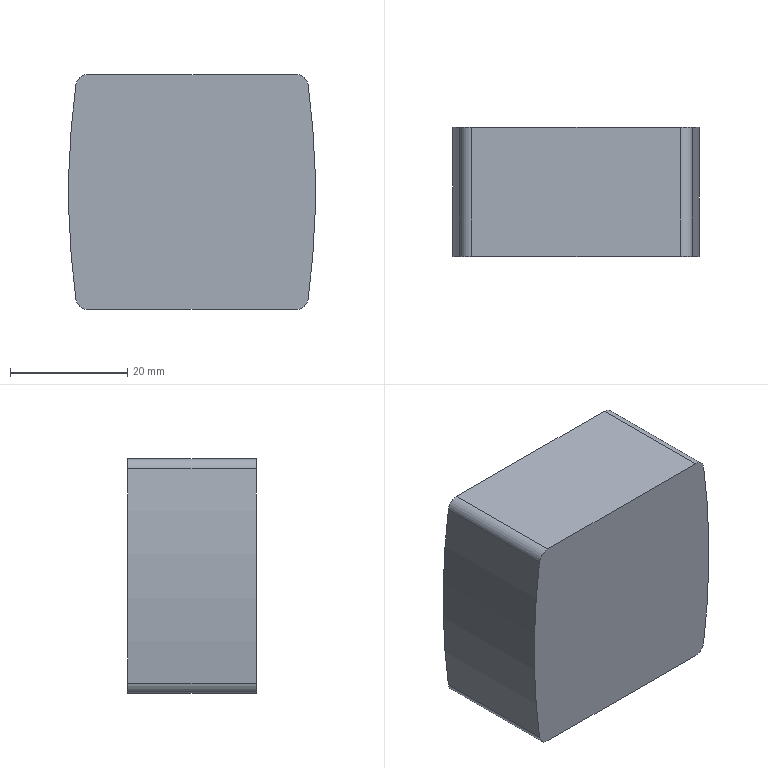Part | SolidWorks | features BaseBody 1 | 1 solid | 12 faces | box 42.009 x 21.95 x 40 mm | volume 35954 mm3 | cylinder 8 | plane 4 | commonest cylinder face diameters 4 x6 268.2 x2
STEP:
#1=CARTESIAN_POINT('',(17.75,69.98,-20.));
#2=VERTEX_POINT('',#1);
#3=CARTESIAN_POINT('',(17.773,69.98,-20.));
#4=VERTEX_POINT('',#3);
#5=CARTESIAN_POINT('',(17.773,69.98,-18.));
#6=DIRECTION('',(0.,-1.,0.));
#7=DIRECTION('',(0.,0.,-1.));
#8=AXIS2_PLACEMENT_3D('',#5,#6,#7);
#9=CIRCLE('',#8,2.);
#10=EDGE_CURVE('',#2,#4,#9,.T.);
#11=ORIENTED_EDGE('',*,*,#10,.T.);
#12=CARTESIAN_POINT('',(17.773,48.03,-20.));
#13=VERTEX_POINT('',#12);
#14=CARTESIAN_POINT('',(17.773,69.98,-20.));
#15=DIRECTION('',(0.,-1.,0.));
#16=VECTOR('',#15,1000.);
#17=LINE('',#14,#16);
#18=EDGE_CURVE('',#4,#13,#17,.T.);
#19=ORIENTED_EDGE('',*,*,#18,.T.);
#20=CARTESIAN_POINT('',(17.75,48.03,-20.));
#21=VERTEX_POINT('',#20);
#22=CARTESIAN_POINT('',(17.773,48.03,-18.));
#23=DIRECTION('',(0.,-1.,0.));
#24=DIRECTION('',(0.,0.,-1.));
#25=AXIS2_PLACEMENT_3D('',#22,#23,#24);
#26=CIRCLE('',#25,2.);
#27=EDGE_CURVE('',#21,#13,#26,.T.);
#28=ORIENTED_EDGE('',*,*,#27,.F.);
#29=CARTESIAN_POINT('',(17.75,69.98,-20.));
#30=DIRECTION('',(0.,1.,0.));
#31=VECTOR('',#30,1000.);
#32=LINE('',#29,#31);
#33=EDGE_CURVE('',#21,#2,#32,.T.);
#34=ORIENTED_EDGE('',*,*,#33,.T.);
#35=EDGE_LOOP('',(#11,#19,#28,#34));
#36=FACE_OUTER_BOUND('',#35,.T.);
#37=CARTESIAN_POINT('',(17.773,69.98,-18.));
#38=DIRECTION('',(0.,-1.,0.));
#39=DIRECTION('',(0.,0.,-1.));
#40=AXIS2_PLACEMENT_3D('',#37,#38,#39);
#41=CYLINDRICAL_SURFACE('',#40,2.);
#42=ADVANCED_FACE('',(#36),#41,.T.);
#43=CARTESIAN_POINT('',(-19.75,69.98,-18.3));
#44=VERTEX_POINT('',#43);
#45=CARTESIAN_POINT('',(-17.773,69.98,-20.));
#46=VERTEX_POINT('',#45);
#47=CARTESIAN_POINT('',(-17.773,69.98,-18.));
#48=DIRECTION('',(0.,-1.,0.));
#49=DIRECTION('',(0.,0.,-1.));
#50=AXIS2_PLACEMENT_3D('',#47,#48,#49);
#51=CIRCLE('',#50,2.);
#52=EDGE_CURVE('',#44,#46,#51,.T.);
#53=ORIENTED_EDGE('',*,*,#52,.T.);
#54=CARTESIAN_POINT('',(-17.773,48.03,-20.));
#55=VERTEX_POINT('',#54);
#56=CARTESIAN_POINT('',(-17.773,69.98,-20.));
#57=DIRECTION('',(0.,-1.,0.));
#58=VECTOR('',#57,1000.);
#59=LINE('',#56,#58);
#60=EDGE_CURVE('',#46,#55,#59,.T.);
#61=ORIENTED_EDGE('',*,*,#60,.T.);
#62=CARTESIAN_POINT('',(-19.75,48.03,-18.3));
#63=VERTEX_POINT('',#62);
#64=CARTESIAN_POINT('',(-17.773,48.03,-18.));
#65=DIRECTION('',(0.,-1.,0.));
#66=DIRECTION('',(0.,0.,-1.));
#67=AXIS2_PLACEMENT_3D('',#64,#65,#66);
#68=CIRCLE('',#67,2.);
#69=EDGE_CURVE('',#63,#55,#68,.T.);
#70=ORIENTED_EDGE('',*,*,#69,.F.);
#71=CARTESIAN_POINT('',(-19.75,69.98,-18.3));
#72=DIRECTION('',(0.,1.,0.));
#73=VECTOR('',#72,1000.);
#74=LINE('',#71,#73);
#75=EDGE_CURVE('',#63,#44,#74,.T.);
#76=ORIENTED_EDGE('',*,*,#75,.T.);
#77=EDGE_LOOP('',(#53,#61,#70,#76));
#78=FACE_OUTER_BOUND('',#77,.T.);
#79=CARTESIAN_POINT('',(-17.773,69.98,-18.));
#80=DIRECTION('',(0.,-1.,0.));
#81=DIRECTION('',(0.,0.,-1.));
#82=AXIS2_PLACEMENT_3D('',#79,#80,#81);
#83=CYLINDRICAL_SURFACE('',#82,2.);
#84=ADVANCED_FACE('',(#78),#83,.T.);
#85=CARTESIAN_POINT('',(19.75,48.03,-18.3));
#86=VERTEX_POINT('',#85);
#87=CARTESIAN_POINT('',(19.75,48.03,18.3));
#88=VERTEX_POINT('',#87);
#89=CARTESIAN_POINT('',(-113.095,48.03,0.));
#90=DIRECTION('',(0.,-1.,0.));
#91=DIRECTION('',(0.,0.,-1.));
#92=AXIS2_PLACEMENT_3D('',#89,#90,#91);
#93=CIRCLE('',#92,134.1);
#94=EDGE_CURVE('',#86,#88,#93,.T.);
#95=ORIENTED_EDGE('',*,*,#94,.T.);
#96=CARTESIAN_POINT('',(17.75,48.03,20.));
#97=VERTEX_POINT('',#96);
#98=CARTESIAN_POINT('',(17.773,48.03,18.));
#99=DIRECTION('',(0.,-1.,0.));
#100=DIRECTION('',(0.,0.,-1.));
#101=AXIS2_PLACEMENT_3D('',#98,#99,#100);
#102=CIRCLE('',#101,2.);
#103=EDGE_CURVE('',#88,#97,#102,.T.);
#104=ORIENTED_EDGE('',*,*,#103,.T.);
#105=CARTESIAN_POINT('',(-17.75,48.03,20.));
#106=VERTEX_POINT('',#105);
#107=CARTESIAN_POINT('',(0.,48.03,20.));
#108=DIRECTION('',(-1.,0.,0.));
#109=VECTOR('',#108,1000.);
#110=LINE('',#107,#109);
#111=EDGE_CURVE('',#97,#106,#110,.T.);
#112=ORIENTED_EDGE('',*,*,#111,.T.);
#113=CARTESIAN_POINT('',(-19.75,48.03,18.3));
#114=VERTEX_POINT('',#113);
#115=CARTESIAN_POINT('',(-17.773,48.03,18.));
#116=DIRECTION('',(0.,-1.,0.));
#117=DIRECTION('',(0.,0.,-1.));
#118=AXIS2_PLACEMENT_3D('',#115,#116,#117);
#119=CIRCLE('',#118,2.);
#120=EDGE_CURVE('',#106,#114,#119,.T.);
#121=ORIENTED_EDGE('',*,*,#120,.T.);
#122=CARTESIAN_POINT('',(113.095,48.03,0.));
#123=DIRECTION('',(0.,-1.,0.));
#124=DIRECTION('',(0.,0.,-1.));
#125=AXIS2_PLACEMENT_3D('',#122,#123,#124);
#126=CIRCLE('',#125,134.1);
#127=EDGE_CURVE('',#114,#63,#126,.T.);
#128=ORIENTED_EDGE('',*,*,#127,.T.);
#129=ORIENTED_EDGE('',*,*,#69,.T.);
#130=CARTESIAN_POINT('',(-17.75,48.03,-20.));
#131=VERTEX_POINT('',#130);
#132=CARTESIAN_POINT('',(-17.773,48.03,-18.));
#133=DIRECTION('',(0.,-1.,0.));
#134=DIRECTION('',(0.,0.,-1.));
#135=AXIS2_PLACEMENT_3D('',#132,#133,#134);
#136=CIRCLE('',#135,2.);
#137=EDGE_CURVE('',#55,#131,#136,.T.);
#138=ORIENTED_EDGE('',*,*,#137,.T.);
#139=CARTESIAN_POINT('',(0.,48.03,-20.));
#140=DIRECTION('',(1.,0.,0.));
#141=VECTOR('',#140,1000.);
#142=LINE('',#139,#141);
#143=EDGE_CURVE('',#131,#21,#142,.T.);
#144=ORIENTED_EDGE('',*,*,#143,.T.);
#145=ORIENTED_EDGE('',*,*,#27,.T.);
#146=CARTESIAN_POINT('',(17.773,48.03,-18.));
#147=DIRECTION('',(0.,-1.,0.));
#148=DIRECTION('',(0.,0.,-1.));
#149=AXIS2_PLACEMENT_3D('',#146,#147,#148);
#150=CIRCLE('',#149,2.);
#151=EDGE_CURVE('',#13,#86,#150,.T.);
#152=ORIENTED_EDGE('',*,*,#151,.T.);
#153=EDGE_LOOP('',(#95,#104,#112,#121,#128,#129,#138,#144,#145,#152));
#154=FACE_OUTER_BOUND('',#153,.T.);
#155=CARTESIAN_POINT('',(0.,48.03,0.));
#156=DIRECTION('',(0.,-1.,0.));
#157=DIRECTION('',(0.,0.,-1.));
#158=AXIS2_PLACEMENT_3D('',#155,#156,#157);
#159=PLANE('',#158);
#160=ADVANCED_FACE('',(#154),#159,.T.);
#161=CARTESIAN_POINT('',(19.75,69.98,18.3));
#162=VERTEX_POINT('',#161);
#163=CARTESIAN_POINT('',(17.75,69.98,20.));
#164=VERTEX_POINT('',#163);
#165=CARTESIAN_POINT('',(17.773,69.98,18.));
#166=DIRECTION('',(0.,-1.,0.));
#167=DIRECTION('',(0.,0.,-1.));
#168=AXIS2_PLACEMENT_3D('',#165,#166,#167);
#169=CIRCLE('',#168,2.);
#170=EDGE_CURVE('',#162,#164,#169,.T.);
#171=ORIENTED_EDGE('',*,*,#170,.T.);
#172=CARTESIAN_POINT('',(17.75,69.98,20.));
#173=DIRECTION('',(0.,-1.,0.));
#174=VECTOR('',#173,1000.);
#175=LINE('',#172,#174);
#176=EDGE_CURVE('',#164,#97,#175,.T.);
#177=ORIENTED_EDGE('',*,*,#176,.T.);
#178=ORIENTED_EDGE('',*,*,#103,.F.);
#179=CARTESIAN_POINT('',(19.75,69.98,18.3));
#180=DIRECTION('',(0.,1.,0.));
#181=VECTOR('',#180,1000.);
#182=LINE('',#179,#181);
#183=EDGE_CURVE('',#88,#162,#182,.T.);
#184=ORIENTED_EDGE('',*,*,#183,.T.);
#185=EDGE_LOOP('',(#171,#177,#178,#184));
#186=FACE_OUTER_BOUND('',#185,.T.);
#187=CARTESIAN_POINT('',(17.773,69.98,18.));
#188=DIRECTION('',(0.,-1.,0.));
#189=DIRECTION('',(0.,0.,-1.));
#190=AXIS2_PLACEMENT_3D('',#187,#188,#189);
#191=CYLINDRICAL_SURFACE('',#190,2.);
#192=ADVANCED_FACE('',(#186),#191,.T.);
#193=CARTESIAN_POINT('',(19.75,69.98,-18.3));
#194=VERTEX_POINT('',#193);
#195=CARTESIAN_POINT('',(-113.095,69.98,0.));
#196=DIRECTION('',(0.,-1.,0.));
#197=DIRECTION('',(0.,0.,-1.));
#198=AXIS2_PLACEMENT_3D('',#195,#196,#197);
#199=CIRCLE('',#198,134.1);
#200=EDGE_CURVE('',#194,#162,#199,.T.);
#201=ORIENTED_EDGE('',*,*,#200,.T.);
#202=ORIENTED_EDGE('',*,*,#183,.F.);
#203=ORIENTED_EDGE('',*,*,#94,.F.);
#204=CARTESIAN_POINT('',(19.75,69.98,-18.3));
#205=DIRECTION('',(0.,1.,0.));
#206=VECTOR('',#205,1000.);
#207=LINE('',#204,#206);
#208=EDGE_CURVE('',#86,#194,#207,.T.);
#209=ORIENTED_EDGE('',*,*,#208,.T.);
#210=EDGE_LOOP('',(#201,#202,#203,#209));
#211=FACE_OUTER_BOUND('',#210,.T.);
#212=CARTESIAN_POINT('',(-113.095,69.98,0.));
#213=DIRECTION('',(0.,-1.,0.));
#214=DIRECTION('',(0.,0.,-1.));
#215=AXIS2_PLACEMENT_3D('',#212,#213,#214);
#216=CYLINDRICAL_SURFACE('',#215,134.1);
#217=ADVANCED_FACE('',(#211),#216,.T.);
#218=ORIENTED_EDGE('',*,*,#18,.F.);
#219=CARTESIAN_POINT('',(17.773,69.98,-18.));
#220=DIRECTION('',(0.,-1.,0.));
#221=DIRECTION('',(0.,0.,-1.));
#222=AXIS2_PLACEMENT_3D('',#219,#220,#221);
#223=CIRCLE('',#222,2.);
#224=EDGE_CURVE('',#4,#194,#223,.T.);
#225=ORIENTED_EDGE('',*,*,#224,.T.);
#226=ORIENTED_EDGE('',*,*,#208,.F.);
#227=ORIENTED_EDGE('',*,*,#151,.F.);
#228=EDGE_LOOP('',(#218,#225,#226,#227));
#229=FACE_OUTER_BOUND('',#228,.T.);
#230=CARTESIAN_POINT('',(17.773,69.98,-18.));
#231=DIRECTION('',(0.,-1.,0.));
#232=DIRECTION('',(0.,0.,-1.));
#233=AXIS2_PLACEMENT_3D('',#230,#231,#232);
#234=CYLINDRICAL_SURFACE('',#233,2.);
#235=ADVANCED_FACE('',(#229),#234,.T.);
#236=CARTESIAN_POINT('',(-17.75,69.98,-20.));
#237=VERTEX_POINT('',#236);
#238=CARTESIAN_POINT('',(0.,69.98,-20.));
#239=DIRECTION('',(1.,0.,0.));
#240=VECTOR('',#239,1000.);
#241=LINE('',#238,#240);
#242=EDGE_CURVE('',#237,#2,#241,.T.);
#243=ORIENTED_EDGE('',*,*,#242,.T.);
#244=ORIENTED_EDGE('',*,*,#33,.F.);
#245=ORIENTED_EDGE('',*,*,#143,.F.);
#246=CARTESIAN_POINT('',(-17.75,69.98,-20.));
#247=DIRECTION('',(0.,1.,0.));
#248=VECTOR('',#247,1000.);
#249=LINE('',#246,#248);
#250=EDGE_CURVE('',#131,#237,#249,.T.);
#251=ORIENTED_EDGE('',*,*,#250,.T.);
#252=EDGE_LOOP('',(#243,#244,#245,#251));
#253=FACE_OUTER_BOUND('',#252,.T.);
#254=CARTESIAN_POINT('',(0.,69.98,-20.));
#255=DIRECTION('',(0.,0.,-1.));
#256=DIRECTION('',(-1.,0.,0.));
#257=AXIS2_PLACEMENT_3D('',#254,#255,#256);
#258=PLANE('',#257);
#259=ADVANCED_FACE('',(#253),#258,.T.);
#260=ORIENTED_EDGE('',*,*,#60,.F.);
#261=CARTESIAN_POINT('',(-17.773,69.98,-18.));
#262=DIRECTION('',(0.,-1.,0.));
#263=DIRECTION('',(0.,0.,-1.));
#264=AXIS2_PLACEMENT_3D('',#261,#262,#263);
#265=CIRCLE('',#264,2.);
#266=EDGE_CURVE('',#46,#237,#265,.T.);
#267=ORIENTED_EDGE('',*,*,#266,.T.);
#268=ORIENTED_EDGE('',*,*,#250,.F.);
#269=ORIENTED_EDGE('',*,*,#137,.F.);
#270=EDGE_LOOP('',(#260,#267,#268,#269));
#271=FACE_OUTER_BOUND('',#270,.T.);
#272=CARTESIAN_POINT('',(-17.773,69.98,-18.));
#273=DIRECTION('',(0.,-1.,0.));
#274=DIRECTION('',(0.,0.,-1.));
#275=AXIS2_PLACEMENT_3D('',#272,#273,#274);
#276=CYLINDRICAL_SURFACE('',#275,2.);
#277=ADVANCED_FACE('',(#271),#276,.T.);
#278=CARTESIAN_POINT('',(-19.75,69.98,18.3));
#279=VERTEX_POINT('',#278);
#280=CARTESIAN_POINT('',(113.095,69.98,0.));
#281=DIRECTION('',(0.,-1.,0.));
#282=DIRECTION('',(0.,0.,-1.));
#283=AXIS2_PLACEMENT_3D('',#280,#281,#282);
#284=CIRCLE('',#283,134.1);
#285=EDGE_CURVE('',#279,#44,#284,.T.);
#286=ORIENTED_EDGE('',*,*,#285,.T.);
#287=ORIENTED_EDGE('',*,*,#75,.F.);
#288=ORIENTED_EDGE('',*,*,#127,.F.);
#289=CARTESIAN_POINT('',(-19.75,69.98,18.3));
#290=DIRECTION('',(0.,1.,0.));
#291=VECTOR('',#290,1000.);
#292=LINE('',#289,#291);
#293=EDGE_CURVE('',#114,#279,#292,.T.);
#294=ORIENTED_EDGE('',*,*,#293,.T.);
#295=EDGE_LOOP('',(#286,#287,#288,#294));
#296=FACE_OUTER_BOUND('',#295,.T.);
#297=CARTESIAN_POINT('',(113.095,69.98,0.));
#298=DIRECTION('',(0.,-1.,0.));
#299=DIRECTION('',(0.,0.,-1.));
#300=AXIS2_PLACEMENT_3D('',#297,#298,#299);
#301=CYLINDRICAL_SURFACE('',#300,134.1);
#302=ADVANCED_FACE('',(#296),#301,.T.);
#303=CARTESIAN_POINT('',(-17.75,69.98,20.));
#304=VERTEX_POINT('',#303);
#305=CARTESIAN_POINT('',(-17.773,69.98,18.));
#306=DIRECTION('',(0.,-1.,0.));
#307=DIRECTION('',(0.,0.,-1.));
#308=AXIS2_PLACEMENT_3D('',#305,#306,#307);
#309=CIRCLE('',#308,2.);
#310=EDGE_CURVE('',#304,#279,#309,.T.);
#311=ORIENTED_EDGE('',*,*,#310,.T.);
#312=ORIENTED_EDGE('',*,*,#293,.F.);
#313=ORIENTED_EDGE('',*,*,#120,.F.);
#314=CARTESIAN_POINT('',(-17.75,69.98,20.));
#315=DIRECTION('',(0.,1.,0.));
#316=VECTOR('',#315,1000.);
#317=LINE('',#314,#316);
#318=EDGE_CURVE('',#106,#304,#317,.T.);
#319=ORIENTED_EDGE('',*,*,#318,.T.);
#320=EDGE_LOOP('',(#311,#312,#313,#319));
#321=FACE_OUTER_BOUND('',#320,.T.);
#322=CARTESIAN_POINT('',(-17.773,69.98,18.));
#323=DIRECTION('',(0.,-1.,0.));
#324=DIRECTION('',(0.,0.,-1.));
#325=AXIS2_PLACEMENT_3D('',#322,#323,#324);
#326=CYLINDRICAL_SURFACE('',#325,2.);
#327=ADVANCED_FACE('',(#321),#326,.T.);
#328=CARTESIAN_POINT('',(8.875,69.98,20.));
#329=DIRECTION('',(-1.,0.,0.));
#330=VECTOR('',#329,1000.);
#331=LINE('',#328,#330);
#332=EDGE_CURVE('',#164,#304,#331,.T.);
#333=ORIENTED_EDGE('',*,*,#332,.T.);
#334=ORIENTED_EDGE('',*,*,#318,.F.);
#335=ORIENTED_EDGE('',*,*,#111,.F.);
#336=ORIENTED_EDGE('',*,*,#176,.F.);
#337=EDGE_LOOP('',(#333,#334,#335,#336));
#338=FACE_OUTER_BOUND('',#337,.T.);
#339=CARTESIAN_POINT('',(8.875,69.98,20.));
#340=DIRECTION('',(0.,0.,1.));
#341=DIRECTION('',(1.,0.,0.));
#342=AXIS2_PLACEMENT_3D('',#339,#340,#341);
#343=PLANE('',#342);
#344=ADVANCED_FACE('',(#338),#343,.T.);
#345=ORIENTED_EDGE('',*,*,#170,.F.);
#346=ORIENTED_EDGE('',*,*,#200,.F.);
#347=ORIENTED_EDGE('',*,*,#224,.F.);
#348=ORIENTED_EDGE('',*,*,#10,.F.);
#349=ORIENTED_EDGE('',*,*,#242,.F.);
#350=ORIENTED_EDGE('',*,*,#266,.F.);
#351=ORIENTED_EDGE('',*,*,#52,.F.);
#352=ORIENTED_EDGE('',*,*,#285,.F.);
#353=ORIENTED_EDGE('',*,*,#310,.F.);
#354=ORIENTED_EDGE('',*,*,#332,.F.);
#355=EDGE_LOOP('',(#345,#346,#347,#348,#349,#350,#351,#352,#353,#354));
#356=FACE_OUTER_BOUND('',#355,.T.);
#357=CARTESIAN_POINT('',(0.,69.98,0.));
#358=DIRECTION('',(0.,-1.,0.));
#359=DIRECTION('',(0.,0.,-1.));
#360=AXIS2_PLACEMENT_3D('',#357,#358,#359);
#361=PLANE('',#360);
#362=ADVANCED_FACE('',(#356),#361,.F.);
#363=CLOSED_SHELL('',(#42,#84,#160,#192,#217,#235,#259,#277,#302,#327,#344,#362));
#364=MANIFOLD_SOLID_BREP('',#363);
#365=CARTESIAN_POINT('',(0.,0.,0.));
#366=DIRECTION('',(0.,0.,1.));
#367=DIRECTION('',(1.,0.,0.));
#368=AXIS2_PLACEMENT_3D('',#365,#366,#367);
#369=(LENGTH_UNIT()NAMED_UNIT(*)SI_UNIT(.MILLI.,.METRE.));
#370=UNCERTAINTY_MEASURE_WITH_UNIT(LENGTH_MEASURE(0.00001),#369,'','');
#371=(NAMED_UNIT(*)PLANE_ANGLE_UNIT()SI_UNIT($,.RADIAN.));
#372=(NAMED_UNIT(*)SI_UNIT($,.STERADIAN.)SOLID_ANGLE_UNIT());
#373=(GEOMETRIC_REPRESENTATION_CONTEXT(3)GLOBAL_UNCERTAINTY_ASSIGNED_CONTEXT((#370))GLOBAL_UNIT_ASSIGNED_CONTEXT((#369,#371,#372))REPRESENTATION_CONTEXT('',''));
#374=ADVANCED_BREP_SHAPE_REPRESENTATION('',(#364,#368),#373);